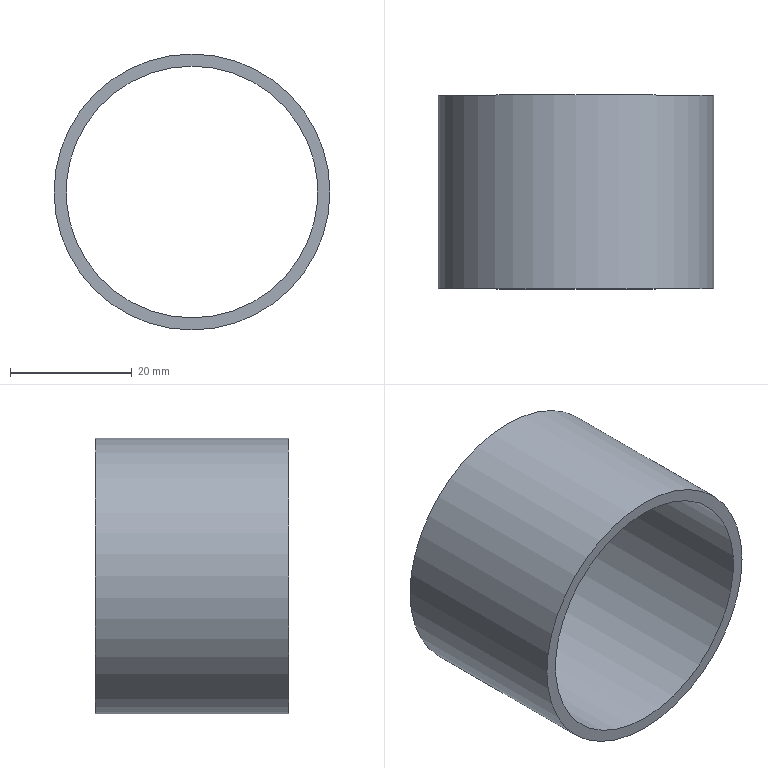Part | NX | features MG0330 trunion parts 24(trunion group) 2 | 1 solid | 4 faces | box 45.248 x 31.75 x 45.248 mm | volume 8571 mm3 | cylinder 2 | plane 2 | commonest cylinder face diameters 41.275 x1 45.248 x1
STEP:
#1=CARTESIAN_POINT('',(0.,166.707,-22.624));
#2=VERTEX_POINT('',#1);
#3=CARTESIAN_POINT('',(0.,166.707,0.));
#4=DIRECTION('',(0.,-1.,0.));
#5=DIRECTION('',(0.,0.,-1.));
#6=AXIS2_PLACEMENT_3D('',#3,#4,#5);
#7=CIRCLE('',#6,22.624);
#8=EDGE_CURVE('',#2,#2,#7,.T.);
#9=ORIENTED_EDGE('',*,*,#8,.T.);
#10=EDGE_LOOP('',(#9));
#11=FACE_BOUND('',#10,.T.);
#12=CARTESIAN_POINT('',(0.,134.957,-22.624));
#13=VERTEX_POINT('',#12);
#14=CARTESIAN_POINT('',(0.,134.957,0.));
#15=DIRECTION('',(0.,-1.,0.));
#16=DIRECTION('',(0.,0.,-1.));
#17=AXIS2_PLACEMENT_3D('',#14,#15,#16);
#18=CIRCLE('',#17,22.624);
#19=EDGE_CURVE('',#13,#13,#18,.T.);
#20=ORIENTED_EDGE('',*,*,#19,.F.);
#21=EDGE_LOOP('',(#20));
#22=FACE_BOUND('',#21,.T.);
#23=CARTESIAN_POINT('',(0.,0.,0.));
#24=DIRECTION('',(0.,-1.,0.));
#25=DIRECTION('',(0.,0.,-1.));
#26=AXIS2_PLACEMENT_3D('',#23,#24,#25);
#27=CYLINDRICAL_SURFACE('',#26,22.624);
#28=ADVANCED_FACE('',(#11,#22),#27,.T.);
#29=ORIENTED_EDGE('',*,*,#19,.T.);
#30=EDGE_LOOP('',(#29));
#31=FACE_BOUND('',#30,.T.);
#32=CARTESIAN_POINT('',(0.,134.957,-20.637));
#33=VERTEX_POINT('',#32);
#34=CARTESIAN_POINT('',(0.,134.957,0.));
#35=DIRECTION('',(0.,-1.,0.));
#36=DIRECTION('',(0.,0.,-1.));
#37=AXIS2_PLACEMENT_3D('',#34,#35,#36);
#38=CIRCLE('',#37,20.637);
#39=EDGE_CURVE('',#33,#33,#38,.T.);
#40=ORIENTED_EDGE('',*,*,#39,.F.);
#41=EDGE_LOOP('',(#40));
#42=FACE_BOUND('',#41,.T.);
#43=CARTESIAN_POINT('',(22.624,134.957,0.));
#44=DIRECTION('',(0.,-1.,0.));
#45=DIRECTION('',(0.,0.,-1.));
#46=AXIS2_PLACEMENT_3D('',#43,#44,#45);
#47=PLANE('',#46);
#48=ADVANCED_FACE('',(#31,#42),#47,.T.);
#49=ORIENTED_EDGE('',*,*,#39,.T.);
#50=EDGE_LOOP('',(#49));
#51=FACE_BOUND('',#50,.T.);
#52=CARTESIAN_POINT('',(0.,166.707,20.637));
#53=VERTEX_POINT('',#52);
#54=CARTESIAN_POINT('',(0.,166.707,0.));
#55=DIRECTION('',(0.,1.,0.));
#56=DIRECTION('',(0.,0.,1.));
#57=AXIS2_PLACEMENT_3D('',#54,#55,#56);
#58=CIRCLE('',#57,20.637);
#59=EDGE_CURVE('',#53,#53,#58,.F.);
#60=ORIENTED_EDGE('',*,*,#59,.F.);
#61=EDGE_LOOP('',(#60));
#62=FACE_BOUND('',#61,.T.);
#63=CARTESIAN_POINT('',(0.,0.,0.));
#64=DIRECTION('',(0.,-1.,0.));
#65=DIRECTION('',(0.,0.,-1.));
#66=AXIS2_PLACEMENT_3D('',#63,#64,#65);
#67=CYLINDRICAL_SURFACE('',#66,20.637);
#68=ADVANCED_FACE('',(#51,#62),#67,.F.);
#69=ORIENTED_EDGE('',*,*,#59,.T.);
#70=EDGE_LOOP('',(#69));
#71=FACE_BOUND('',#70,.T.);
#72=ORIENTED_EDGE('',*,*,#8,.F.);
#73=EDGE_LOOP('',(#72));
#74=FACE_BOUND('',#73,.T.);
#75=CARTESIAN_POINT('',(22.624,166.707,0.));
#76=DIRECTION('',(0.,1.,0.));
#77=DIRECTION('',(0.,0.,1.));
#78=AXIS2_PLACEMENT_3D('',#75,#76,#77);
#79=PLANE('',#78);
#80=ADVANCED_FACE('',(#71,#74),#79,.T.);
#81=CLOSED_SHELL('',(#28,#48,#68,#80));
#82=MANIFOLD_SOLID_BREP('',#81);
#83=(LENGTH_UNIT()NAMED_UNIT(*)SI_UNIT(.MILLI.,.METRE.));
#84=UNCERTAINTY_MEASURE_WITH_UNIT(LENGTH_MEASURE(0.00001),#83,'','');
#85=(NAMED_UNIT(*)PLANE_ANGLE_UNIT()SI_UNIT($,.RADIAN.));
#86=(NAMED_UNIT(*)SI_UNIT($,.STERADIAN.)SOLID_ANGLE_UNIT());
#87=(GEOMETRIC_REPRESENTATION_CONTEXT(3)GLOBAL_UNCERTAINTY_ASSIGNED_CONTEXT((#84))GLOBAL_UNIT_ASSIGNED_CONTEXT((#83,#85,#86))REPRESENTATION_CONTEXT('',''));
#88=ADVANCED_BREP_SHAPE_REPRESENTATION('',(#82),#87);